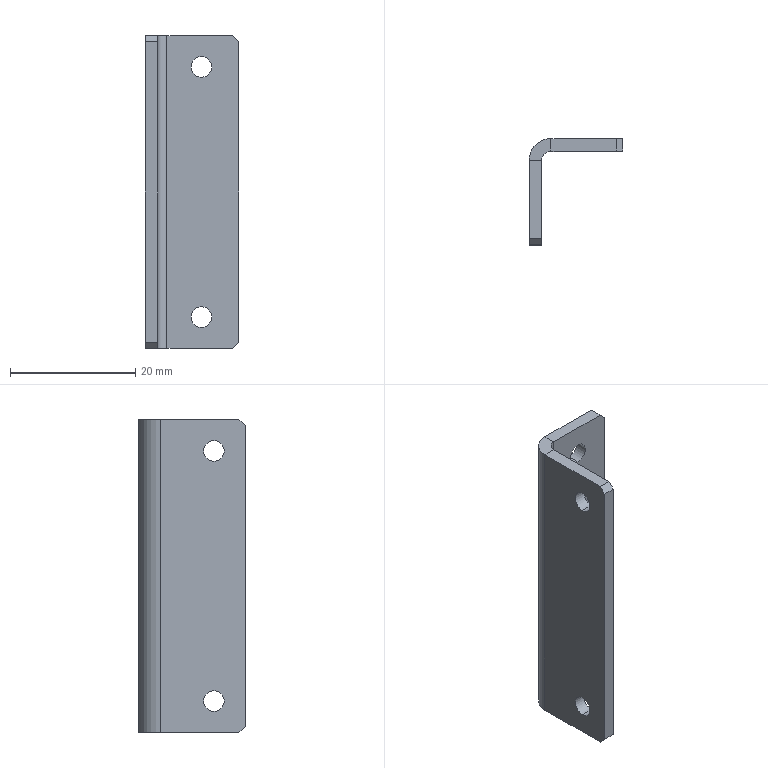Part | SolidWorks | features HoleWzd 2, Chamfer 1, FlatPattern 1, SMBaseFlange 1, SheetMetal 1 | 1 solid | 26 faces | box 15 x 17 x 50 mm | volume 2820 mm3 | plane 16 | cylinder 10 | commonest cylinder face diameters 3.3 x8 3 x1 7 x1
STEP:
#1=CARTESIAN_POINT('',(2.,5.,18.35));
#2=VERTEX_POINT('',#1);
#3=CARTESIAN_POINT('',(2.,5.,21.65));
#4=VERTEX_POINT('',#3);
#5=CARTESIAN_POINT('',(2.,5.,20.));
#6=DIRECTION('',(-1.,0.,0.));
#7=DIRECTION('',(0.,0.,1.));
#8=AXIS2_PLACEMENT_3D('',#5,#6,#7);
#9=CIRCLE('',#8,1.65);
#10=EDGE_CURVE('',#2,#4,#9,.T.);
#11=ORIENTED_EDGE('',*,*,#10,.F.);
#12=CARTESIAN_POINT('',(0.,5.,18.35));
#13=VERTEX_POINT('',#12);
#14=CARTESIAN_POINT('',(0.,5.,18.35));
#15=DIRECTION('',(-1.,0.,0.));
#16=VECTOR('',#15,1000.);
#17=LINE('',#14,#16);
#18=EDGE_CURVE('',#2,#13,#17,.T.);
#19=ORIENTED_EDGE('',*,*,#18,.T.);
#20=CARTESIAN_POINT('',(0.,5.,21.65));
#21=VERTEX_POINT('',#20);
#22=CARTESIAN_POINT('',(0.,5.,20.));
#23=DIRECTION('',(-1.,0.,0.));
#24=DIRECTION('',(0.,0.,1.));
#25=AXIS2_PLACEMENT_3D('',#22,#23,#24);
#26=CIRCLE('',#25,1.65);
#27=EDGE_CURVE('',#13,#21,#26,.T.);
#28=ORIENTED_EDGE('',*,*,#27,.T.);
#29=CARTESIAN_POINT('',(0.,5.,21.65));
#30=DIRECTION('',(-1.,0.,0.));
#31=VECTOR('',#30,1000.);
#32=LINE('',#29,#31);
#33=EDGE_CURVE('',#4,#21,#32,.T.);
#34=ORIENTED_EDGE('',*,*,#33,.F.);
#35=EDGE_LOOP('',(#11,#19,#28,#34));
#36=FACE_OUTER_BOUND('',#35,.T.);
#37=CARTESIAN_POINT('',(0.,5.,20.));
#38=DIRECTION('',(-1.,0.,0.));
#39=DIRECTION('',(0.,0.,1.));
#40=AXIS2_PLACEMENT_3D('',#37,#38,#39);
#41=CYLINDRICAL_SURFACE('',#40,1.65);
#42=ADVANCED_FACE('',(#36),#41,.F.);
#43=CARTESIAN_POINT('',(2.,5.,-21.65));
#44=VERTEX_POINT('',#43);
#45=CARTESIAN_POINT('',(2.,5.,-18.35));
#46=VERTEX_POINT('',#45);
#47=CARTESIAN_POINT('',(2.,5.,-20.));
#48=DIRECTION('',(-1.,0.,0.));
#49=DIRECTION('',(0.,0.,1.));
#50=AXIS2_PLACEMENT_3D('',#47,#48,#49);
#51=CIRCLE('',#50,1.65);
#52=EDGE_CURVE('',#44,#46,#51,.T.);
#53=ORIENTED_EDGE('',*,*,#52,.F.);
#54=CARTESIAN_POINT('',(0.,5.,-21.65));
#55=VERTEX_POINT('',#54);
#56=CARTESIAN_POINT('',(0.,5.,-21.65));
#57=DIRECTION('',(-1.,0.,0.));
#58=VECTOR('',#57,1000.);
#59=LINE('',#56,#58);
#60=EDGE_CURVE('',#44,#55,#59,.T.);
#61=ORIENTED_EDGE('',*,*,#60,.T.);
#62=CARTESIAN_POINT('',(0.,5.,-18.35));
#63=VERTEX_POINT('',#62);
#64=CARTESIAN_POINT('',(0.,5.,-20.));
#65=DIRECTION('',(-1.,0.,0.));
#66=DIRECTION('',(0.,0.,1.));
#67=AXIS2_PLACEMENT_3D('',#64,#65,#66);
#68=CIRCLE('',#67,1.65);
#69=EDGE_CURVE('',#55,#63,#68,.T.);
#70=ORIENTED_EDGE('',*,*,#69,.T.);
#71=CARTESIAN_POINT('',(0.,5.,-18.35));
#72=DIRECTION('',(-1.,0.,0.));
#73=VECTOR('',#72,1000.);
#74=LINE('',#71,#73);
#75=EDGE_CURVE('',#46,#63,#74,.T.);
#76=ORIENTED_EDGE('',*,*,#75,.F.);
#77=EDGE_LOOP('',(#53,#61,#70,#76));
#78=FACE_OUTER_BOUND('',#77,.T.);
#79=CARTESIAN_POINT('',(0.,5.,-20.));
#80=DIRECTION('',(-1.,0.,0.));
#81=DIRECTION('',(0.,0.,1.));
#82=AXIS2_PLACEMENT_3D('',#79,#80,#81);
#83=CYLINDRICAL_SURFACE('',#82,1.65);
#84=ADVANCED_FACE('',(#78),#83,.F.);
#85=CARTESIAN_POINT('',(9.,15.,-21.65));
#86=VERTEX_POINT('',#85);
#87=CARTESIAN_POINT('',(9.,15.,-18.35));
#88=VERTEX_POINT('',#87);
#89=CARTESIAN_POINT('',(9.,15.,-20.));
#90=DIRECTION('',(0.,1.,0.));
#91=DIRECTION('',(0.,0.,1.));
#92=AXIS2_PLACEMENT_3D('',#89,#90,#91);
#93=CIRCLE('',#92,1.65);
#94=EDGE_CURVE('',#86,#88,#93,.T.);
#95=ORIENTED_EDGE('',*,*,#94,.F.);
#96=CARTESIAN_POINT('',(9.,17.,-21.65));
#97=VERTEX_POINT('',#96);
#98=CARTESIAN_POINT('',(9.,17.,-21.65));
#99=DIRECTION('',(0.,1.,0.));
#100=VECTOR('',#99,1000.);
#101=LINE('',#98,#100);
#102=EDGE_CURVE('',#86,#97,#101,.T.);
#103=ORIENTED_EDGE('',*,*,#102,.T.);
#104=CARTESIAN_POINT('',(9.,17.,-18.35));
#105=VERTEX_POINT('',#104);
#106=CARTESIAN_POINT('',(9.,17.,-20.));
#107=DIRECTION('',(0.,1.,0.));
#108=DIRECTION('',(0.,0.,1.));
#109=AXIS2_PLACEMENT_3D('',#106,#107,#108);
#110=CIRCLE('',#109,1.65);
#111=EDGE_CURVE('',#97,#105,#110,.T.);
#112=ORIENTED_EDGE('',*,*,#111,.T.);
#113=CARTESIAN_POINT('',(9.,17.,-18.35));
#114=DIRECTION('',(0.,1.,0.));
#115=VECTOR('',#114,1000.);
#116=LINE('',#113,#115);
#117=EDGE_CURVE('',#88,#105,#116,.T.);
#118=ORIENTED_EDGE('',*,*,#117,.F.);
#119=EDGE_LOOP('',(#95,#103,#112,#118));
#120=FACE_OUTER_BOUND('',#119,.T.);
#121=CARTESIAN_POINT('',(9.,17.,-20.));
#122=DIRECTION('',(0.,1.,0.));
#123=DIRECTION('',(0.,0.,1.));
#124=AXIS2_PLACEMENT_3D('',#121,#122,#123);
#125=CYLINDRICAL_SURFACE('',#124,1.65);
#126=ADVANCED_FACE('',(#120),#125,.F.);
#127=CARTESIAN_POINT('',(9.,15.,18.35));
#128=VERTEX_POINT('',#127);
#129=CARTESIAN_POINT('',(9.,15.,21.65));
#130=VERTEX_POINT('',#129);
#131=CARTESIAN_POINT('',(9.,15.,20.));
#132=DIRECTION('',(0.,1.,0.));
#133=DIRECTION('',(0.,0.,1.));
#134=AXIS2_PLACEMENT_3D('',#131,#132,#133);
#135=CIRCLE('',#134,1.65);
#136=EDGE_CURVE('',#128,#130,#135,.T.);
#137=ORIENTED_EDGE('',*,*,#136,.F.);
#138=CARTESIAN_POINT('',(9.,17.,18.35));
#139=VERTEX_POINT('',#138);
#140=CARTESIAN_POINT('',(9.,17.,18.35));
#141=DIRECTION('',(0.,1.,0.));
#142=VECTOR('',#141,1000.);
#143=LINE('',#140,#142);
#144=EDGE_CURVE('',#128,#139,#143,.T.);
#145=ORIENTED_EDGE('',*,*,#144,.T.);
#146=CARTESIAN_POINT('',(9.,17.,21.65));
#147=VERTEX_POINT('',#146);
#148=CARTESIAN_POINT('',(9.,17.,20.));
#149=DIRECTION('',(0.,1.,0.));
#150=DIRECTION('',(0.,0.,1.));
#151=AXIS2_PLACEMENT_3D('',#148,#149,#150);
#152=CIRCLE('',#151,1.65);
#153=EDGE_CURVE('',#139,#147,#152,.T.);
#154=ORIENTED_EDGE('',*,*,#153,.T.);
#155=CARTESIAN_POINT('',(9.,17.,21.65));
#156=DIRECTION('',(0.,1.,0.));
#157=VECTOR('',#156,1000.);
#158=LINE('',#155,#157);
#159=EDGE_CURVE('',#130,#147,#158,.T.);
#160=ORIENTED_EDGE('',*,*,#159,.F.);
#161=EDGE_LOOP('',(#137,#145,#154,#160));
#162=FACE_OUTER_BOUND('',#161,.T.);
#163=CARTESIAN_POINT('',(9.,17.,20.));
#164=DIRECTION('',(0.,1.,0.));
#165=DIRECTION('',(0.,0.,1.));
#166=AXIS2_PLACEMENT_3D('',#163,#164,#165);
#167=CYLINDRICAL_SURFACE('',#166,1.65);
#168=ADVANCED_FACE('',(#162),#167,.F.);
#169=CARTESIAN_POINT('',(3.5,17.,25.));
#170=VERTEX_POINT('',#169);
#171=CARTESIAN_POINT('',(3.5,15.,25.));
#172=VERTEX_POINT('',#171);
#173=CARTESIAN_POINT('',(3.5,17.,25.));
#174=DIRECTION('',(0.,-1.,0.));
#175=VECTOR('',#174,1000.);
#176=LINE('',#173,#175);
#177=EDGE_CURVE('',#170,#172,#176,.T.);
#178=ORIENTED_EDGE('',*,*,#177,.F.);
#179=CARTESIAN_POINT('',(0.,13.5,25.));
#180=VERTEX_POINT('',#179);
#181=CARTESIAN_POINT('',(3.5,13.5,25.));
#182=DIRECTION('',(0.,0.,-1.));
#183=DIRECTION('',(1.,0.,0.));
#184=AXIS2_PLACEMENT_3D('',#181,#182,#183);
#185=CIRCLE('',#184,3.5);
#186=EDGE_CURVE('',#180,#170,#185,.T.);
#187=ORIENTED_EDGE('',*,*,#186,.F.);
#188=CARTESIAN_POINT('',(2.,13.5,25.));
#189=VERTEX_POINT('',#188);
#190=CARTESIAN_POINT('',(2.,13.5,25.));
#191=DIRECTION('',(-1.,0.,0.));
#192=VECTOR('',#191,1000.);
#193=LINE('',#190,#192);
#194=EDGE_CURVE('',#189,#180,#193,.T.);
#195=ORIENTED_EDGE('',*,*,#194,.F.);
#196=CARTESIAN_POINT('',(3.5,13.5,25.));
#197=DIRECTION('',(0.,0.,-1.));
#198=DIRECTION('',(1.,0.,0.));
#199=AXIS2_PLACEMENT_3D('',#196,#197,#198);
#200=CIRCLE('',#199,1.5);
#201=EDGE_CURVE('',#189,#172,#200,.T.);
#202=ORIENTED_EDGE('',*,*,#201,.T.);
#203=EDGE_LOOP('',(#178,#187,#195,#202));
#204=FACE_OUTER_BOUND('',#203,.T.);
#205=CARTESIAN_POINT('',(3.5,17.,25.));
#206=DIRECTION('',(0.,0.,1.));
#207=DIRECTION('',(1.,0.,0.));
#208=AXIS2_PLACEMENT_3D('',#205,#206,#207);
#209=PLANE('',#208);
#210=ADVANCED_FACE('',(#204),#209,.T.);
#211=CARTESIAN_POINT('',(14.,15.,25.));
#212=VERTEX_POINT('',#211);
#213=CARTESIAN_POINT('',(0.,15.,25.));
#214=DIRECTION('',(1.,0.,0.));
#215=VECTOR('',#214,1000.);
#216=LINE('',#213,#215);
#217=EDGE_CURVE('',#172,#212,#216,.T.);
#218=ORIENTED_EDGE('',*,*,#217,.T.);
#219=CARTESIAN_POINT('',(14.,17.,25.));
#220=VERTEX_POINT('',#219);
#221=CARTESIAN_POINT('',(14.,13.5,25.));
#222=DIRECTION('',(0.,1.,0.));
#223=VECTOR('',#222,1000.);
#224=LINE('',#221,#223);
#225=EDGE_CURVE('',#212,#220,#224,.T.);
#226=ORIENTED_EDGE('',*,*,#225,.T.);
#227=CARTESIAN_POINT('',(0.,17.,25.));
#228=DIRECTION('',(1.,0.,0.));
#229=VECTOR('',#228,1000.);
#230=LINE('',#227,#229);
#231=EDGE_CURVE('',#170,#220,#230,.T.);
#232=ORIENTED_EDGE('',*,*,#231,.F.);
#233=ORIENTED_EDGE('',*,*,#177,.T.);
#234=EDGE_LOOP('',(#218,#226,#232,#233));
#235=FACE_OUTER_BOUND('',#234,.T.);
#236=CARTESIAN_POINT('',(2.,13.5,25.));
#237=DIRECTION('',(0.,0.,1.));
#238=DIRECTION('',(1.,0.,0.));
#239=AXIS2_PLACEMENT_3D('',#236,#237,#238);
#240=PLANE('',#239);
#241=ADVANCED_FACE('',(#235),#240,.T.);
#242=CARTESIAN_POINT('',(0.,13.5,-25.));
#243=VERTEX_POINT('',#242);
#244=CARTESIAN_POINT('',(2.,13.5,-25.));
#245=VERTEX_POINT('',#244);
#246=CARTESIAN_POINT('',(0.,13.5,-25.));
#247=DIRECTION('',(1.,0.,0.));
#248=VECTOR('',#247,1000.);
#249=LINE('',#246,#248);
#250=EDGE_CURVE('',#243,#245,#249,.T.);
#251=ORIENTED_EDGE('',*,*,#250,.F.);
#252=CARTESIAN_POINT('',(3.5,17.,-25.));
#253=VERTEX_POINT('',#252);
#254=CARTESIAN_POINT('',(3.5,13.5,-25.));
#255=DIRECTION('',(0.,0.,-1.));
#256=DIRECTION('',(1.,0.,0.));
#257=AXIS2_PLACEMENT_3D('',#254,#255,#256);
#258=CIRCLE('',#257,3.5);
#259=EDGE_CURVE('',#243,#253,#258,.T.);
#260=ORIENTED_EDGE('',*,*,#259,.T.);
#261=CARTESIAN_POINT('',(3.5,15.,-25.));
#262=VERTEX_POINT('',#261);
#263=CARTESIAN_POINT('',(3.5,15.,-25.));
#264=DIRECTION('',(0.,1.,0.));
#265=VECTOR('',#264,1000.);
#266=LINE('',#263,#265);
#267=EDGE_CURVE('',#262,#253,#266,.T.);
#268=ORIENTED_EDGE('',*,*,#267,.F.);
#269=CARTESIAN_POINT('',(3.5,13.5,-25.));
#270=DIRECTION('',(0.,0.,-1.));
#271=DIRECTION('',(1.,0.,0.));
#272=AXIS2_PLACEMENT_3D('',#269,#270,#271);
#273=CIRCLE('',#272,1.5);
#274=EDGE_CURVE('',#245,#262,#273,.T.);
#275=ORIENTED_EDGE('',*,*,#274,.F.);
#276=EDGE_LOOP('',(#251,#260,#268,#275));
#277=FACE_OUTER_BOUND('',#276,.T.);
#278=CARTESIAN_POINT('',(0.,13.5,-25.));
#279=DIRECTION('',(0.,0.,-1.));
#280=DIRECTION('',(-1.,0.,0.));
#281=AXIS2_PLACEMENT_3D('',#278,#279,#280);
#282=PLANE('',#281);
#283=ADVANCED_FACE('',(#277),#282,.T.);
#284=CARTESIAN_POINT('',(2.,1.,-25.));
#285=VERTEX_POINT('',#284);
#286=CARTESIAN_POINT('',(2.,0.,-25.));
#287=DIRECTION('',(0.,1.,0.));
#288=VECTOR('',#287,1000.);
#289=LINE('',#286,#288);
#290=EDGE_CURVE('',#285,#245,#289,.T.);
#291=ORIENTED_EDGE('',*,*,#290,.F.);
#292=CARTESIAN_POINT('',(0.,1.,-25.));
#293=VERTEX_POINT('',#292);
#294=CARTESIAN_POINT('',(3.5,1.,-25.));
#295=DIRECTION('',(-1.,0.,0.));
#296=VECTOR('',#295,1000.);
#297=LINE('',#294,#296);
#298=EDGE_CURVE('',#285,#293,#297,.T.);
#299=ORIENTED_EDGE('',*,*,#298,.T.);
#300=CARTESIAN_POINT('',(0.,0.,-25.));
#301=DIRECTION('',(0.,1.,0.));
#302=VECTOR('',#301,1000.);
#303=LINE('',#300,#302);
#304=EDGE_CURVE('',#293,#243,#303,.T.);
#305=ORIENTED_EDGE('',*,*,#304,.T.);
#306=ORIENTED_EDGE('',*,*,#250,.T.);
#307=EDGE_LOOP('',(#291,#299,#305,#306));
#308=FACE_OUTER_BOUND('',#307,.T.);
#309=CARTESIAN_POINT('',(3.5,15.,-25.));
#310=DIRECTION('',(0.,0.,-1.));
#311=DIRECTION('',(-1.,0.,0.));
#312=AXIS2_PLACEMENT_3D('',#309,#310,#311);
#313=PLANE('',#312);
#314=ADVANCED_FACE('',(#308),#313,.T.);
#315=CARTESIAN_POINT('',(9.,15.,-20.));
#316=DIRECTION('',(0.,1.,0.));
#317=DIRECTION('',(0.,0.,1.));
#318=AXIS2_PLACEMENT_3D('',#315,#316,#317);
#319=CIRCLE('',#318,1.65);
#320=EDGE_CURVE('',#88,#86,#319,.T.);
#321=ORIENTED_EDGE('',*,*,#320,.T.);
#322=ORIENTED_EDGE('',*,*,#94,.T.);
#323=EDGE_LOOP('',(#321,#322));
#324=FACE_BOUND('',#323,.T.);
#325=CARTESIAN_POINT('',(9.,15.,20.));
#326=DIRECTION('',(0.,1.,0.));
#327=DIRECTION('',(0.,0.,1.));
#328=AXIS2_PLACEMENT_3D('',#325,#326,#327);
#329=CIRCLE('',#328,1.65);
#330=EDGE_CURVE('',#130,#128,#329,.T.);
#331=ORIENTED_EDGE('',*,*,#330,.T.);
#332=ORIENTED_EDGE('',*,*,#136,.T.);
#333=EDGE_LOOP('',(#331,#332));
#334=FACE_BOUND('',#333,.T.);
#335=CARTESIAN_POINT('',(14.,15.,-25.));
#336=VERTEX_POINT('',#335);
#337=CARTESIAN_POINT('',(0.,15.,-25.));
#338=DIRECTION('',(1.,0.,0.));
#339=VECTOR('',#338,1000.);
#340=LINE('',#337,#339);
#341=EDGE_CURVE('',#262,#336,#340,.T.);
#342=ORIENTED_EDGE('',*,*,#341,.T.);
#343=CARTESIAN_POINT('',(15.,15.,-24.));
#344=VERTEX_POINT('',#343);
#345=CARTESIAN_POINT('',(14.,15.,-25.));
#346=DIRECTION('',(0.7071,0.,0.7071));
#347=VECTOR('',#346,1000.);
#348=LINE('',#345,#347);
#349=EDGE_CURVE('',#336,#344,#348,.T.);
#350=ORIENTED_EDGE('',*,*,#349,.T.);
#351=CARTESIAN_POINT('',(15.,15.,24.));
#352=VERTEX_POINT('',#351);
#353=CARTESIAN_POINT('',(15.,15.,25.));
#354=DIRECTION('',(0.,0.,-1.));
#355=VECTOR('',#354,1000.);
#356=LINE('',#353,#355);
#357=EDGE_CURVE('',#352,#344,#356,.T.);
#358=ORIENTED_EDGE('',*,*,#357,.F.);
#359=CARTESIAN_POINT('',(15.,15.,24.));
#360=DIRECTION('',(-0.7071,0.,0.7071));
#361=VECTOR('',#360,1000.);
#362=LINE('',#359,#361);
#363=EDGE_CURVE('',#352,#212,#362,.T.);
#364=ORIENTED_EDGE('',*,*,#363,.T.);
#365=ORIENTED_EDGE('',*,*,#217,.F.);
#366=CARTESIAN_POINT('',(3.5,15.,25.));
#367=DIRECTION('',(0.,0.,-1.));
#368=VECTOR('',#367,1000.);
#369=LINE('',#366,#368);
#370=EDGE_CURVE('',#172,#262,#369,.T.);
#371=ORIENTED_EDGE('',*,*,#370,.T.);
#372=EDGE_LOOP('',(#342,#350,#358,#364,#365,#371));
#373=FACE_OUTER_BOUND('',#372,.T.);
#374=CARTESIAN_POINT('',(0.,15.,25.));
#375=DIRECTION('',(0.,1.,0.));
#376=DIRECTION('',(0.,0.,1.));
#377=AXIS2_PLACEMENT_3D('',#374,#375,#376);
#378=PLANE('',#377);
#379=ADVANCED_FACE('',(#324,#334,#373),#378,.F.);
#380=ORIENTED_EDGE('',*,*,#357,.T.);
#381=CARTESIAN_POINT('',(15.,17.,-24.));
#382=VERTEX_POINT('',#381);
#383=CARTESIAN_POINT('',(15.,17.,-24.));
#384=DIRECTION('',(0.,1.,0.));
#385=VECTOR('',#384,1000.);
#386=LINE('',#383,#385);
#387=EDGE_CURVE('',#344,#382,#386,.T.);
#388=ORIENTED_EDGE('',*,*,#387,.T.);
#389=CARTESIAN_POINT('',(15.,17.,24.));
#390=VERTEX_POINT('',#389);
#391=CARTESIAN_POINT('',(15.,17.,25.));
#392=DIRECTION('',(0.,0.,-1.));
#393=VECTOR('',#392,1000.);
#394=LINE('',#391,#393);
#395=EDGE_CURVE('',#390,#382,#394,.T.);
#396=ORIENTED_EDGE('',*,*,#395,.F.);
#397=CARTESIAN_POINT('',(15.,17.,24.));
#398=DIRECTION('',(0.,-1.,0.));
#399=VECTOR('',#398,1000.);
#400=LINE('',#397,#399);
#401=EDGE_CURVE('',#390,#352,#400,.T.);
#402=ORIENTED_EDGE('',*,*,#401,.T.);
#403=EDGE_LOOP('',(#380,#388,#396,#402));
#404=FACE_OUTER_BOUND('',#403,.T.);
#405=CARTESIAN_POINT('',(15.,17.,25.));
#406=DIRECTION('',(1.,0.,0.));
#407=DIRECTION('',(0.,0.,-1.));
#408=AXIS2_PLACEMENT_3D('',#405,#406,#407);
#409=PLANE('',#408);
#410=ADVANCED_FACE('',(#404),#409,.T.);
#411=CARTESIAN_POINT('',(9.,17.,-20.));
#412=DIRECTION('',(0.,1.,0.));
#413=DIRECTION('',(0.,0.,1.));
#414=AXIS2_PLACEMENT_3D('',#411,#412,#413);
#415=CIRCLE('',#414,1.65);
#416=EDGE_CURVE('',#105,#97,#415,.T.);
#417=ORIENTED_EDGE('',*,*,#416,.F.);
#418=ORIENTED_EDGE('',*,*,#111,.F.);
#419=EDGE_LOOP('',(#417,#418));
#420=FACE_BOUND('',#419,.T.);
#421=CARTESIAN_POINT('',(9.,17.,20.));
#422=DIRECTION('',(0.,1.,0.));
#423=DIRECTION('',(0.,0.,1.));
#424=AXIS2_PLACEMENT_3D('',#421,#422,#423);
#425=CIRCLE('',#424,1.65);
#426=EDGE_CURVE('',#147,#139,#425,.T.);
#427=ORIENTED_EDGE('',*,*,#426,.F.);
#428=ORIENTED_EDGE('',*,*,#153,.F.);
#429=EDGE_LOOP('',(#427,#428));
#430=FACE_BOUND('',#429,.T.);
#431=ORIENTED_EDGE('',*,*,#395,.T.);
#432=CARTESIAN_POINT('',(14.,17.,-25.));
#433=VERTEX_POINT('',#432);
#434=CARTESIAN_POINT('',(32.,17.,-7.));
#435=DIRECTION('',(-0.7071,0.,-0.7071));
#436=VECTOR('',#435,1000.);
#437=LINE('',#434,#436);
#438=EDGE_CURVE('',#382,#433,#437,.T.);
#439=ORIENTED_EDGE('',*,*,#438,.T.);
#440=CARTESIAN_POINT('',(0.,17.,-25.));
#441=DIRECTION('',(1.,0.,0.));
#442=VECTOR('',#441,1000.);
#443=LINE('',#440,#442);
#444=EDGE_CURVE('',#253,#433,#443,.T.);
#445=ORIENTED_EDGE('',*,*,#444,.F.);
#446=CARTESIAN_POINT('',(3.5,17.,25.));
#447=DIRECTION('',(0.,0.,-1.));
#448=VECTOR('',#447,1000.);
#449=LINE('',#446,#448);
#450=EDGE_CURVE('',#170,#253,#449,.T.);
#451=ORIENTED_EDGE('',*,*,#450,.F.);
#452=ORIENTED_EDGE('',*,*,#231,.T.);
#453=CARTESIAN_POINT('',(7.,17.,32.));
#454=DIRECTION('',(0.7071,0.,-0.7071));
#455=VECTOR('',#454,1000.);
#456=LINE('',#453,#455);
#457=EDGE_CURVE('',#220,#390,#456,.T.);
#458=ORIENTED_EDGE('',*,*,#457,.T.);
#459=EDGE_LOOP('',(#431,#439,#445,#451,#452,#458));
#460=FACE_OUTER_BOUND('',#459,.T.);
#461=CARTESIAN_POINT('',(0.,17.,25.));
#462=DIRECTION('',(0.,1.,0.));
#463=DIRECTION('',(0.,0.,1.));
#464=AXIS2_PLACEMENT_3D('',#461,#462,#463);
#465=PLANE('',#464);
#466=ADVANCED_FACE('',(#420,#430,#460),#465,.T.);
#467=ORIENTED_EDGE('',*,*,#259,.F.);
#468=CARTESIAN_POINT('',(0.,13.5,25.));
#469=DIRECTION('',(0.,0.,-1.));
#470=VECTOR('',#469,1000.);
#471=LINE('',#468,#470);
#472=EDGE_CURVE('',#180,#243,#471,.T.);
#473=ORIENTED_EDGE('',*,*,#472,.F.);
#474=ORIENTED_EDGE('',*,*,#186,.T.);
#475=ORIENTED_EDGE('',*,*,#450,.T.);
#476=EDGE_LOOP('',(#467,#473,#474,#475));
#477=FACE_OUTER_BOUND('',#476,.T.);
#478=CARTESIAN_POINT('',(3.5,13.5,25.));
#479=DIRECTION('',(0.,0.,-1.));
#480=DIRECTION('',(-1.,0.,0.));
#481=AXIS2_PLACEMENT_3D('',#478,#479,#480);
#482=CYLINDRICAL_SURFACE('',#481,3.5);
#483=ADVANCED_FACE('',(#477),#482,.T.);
#484=CARTESIAN_POINT('',(0.,5.,20.));
#485=DIRECTION('',(-1.,0.,0.));
#486=DIRECTION('',(0.,0.,1.));
#487=AXIS2_PLACEMENT_3D('',#484,#485,#486);
#488=CIRCLE('',#487,1.65);
#489=EDGE_CURVE('',#21,#13,#488,.T.);
#490=ORIENTED_EDGE('',*,*,#489,.F.);
#491=ORIENTED_EDGE('',*,*,#27,.F.);
#492=EDGE_LOOP('',(#490,#491));
#493=FACE_BOUND('',#492,.T.);
#494=CARTESIAN_POINT('',(0.,5.,-20.));
#495=DIRECTION('',(-1.,0.,0.));
#496=DIRECTION('',(0.,0.,1.));
#497=AXIS2_PLACEMENT_3D('',#494,#495,#496);
#498=CIRCLE('',#497,1.65);
#499=EDGE_CURVE('',#63,#55,#498,.T.);
#500=ORIENTED_EDGE('',*,*,#499,.F.);
#501=ORIENTED_EDGE('',*,*,#69,.F.);
#502=EDGE_LOOP('',(#500,#501));
#503=FACE_BOUND('',#502,.T.);
#504=ORIENTED_EDGE('',*,*,#304,.F.);
#505=CARTESIAN_POINT('',(0.,0.,-24.));
#506=VERTEX_POINT('',#505);
#507=CARTESIAN_POINT('',(0.,-24.5,0.5));
#508=DIRECTION('',(0.,-0.7071,0.7071));
#509=VECTOR('',#508,1000.);
#510=LINE('',#507,#509);
#511=EDGE_CURVE('',#293,#506,#510,.T.);
#512=ORIENTED_EDGE('',*,*,#511,.T.);
#513=CARTESIAN_POINT('',(0.,0.,24.));
#514=VERTEX_POINT('',#513);
#515=CARTESIAN_POINT('',(0.,0.,25.));
#516=DIRECTION('',(0.,0.,-1.));
#517=VECTOR('',#516,1000.);
#518=LINE('',#515,#517);
#519=EDGE_CURVE('',#514,#506,#518,.T.);
#520=ORIENTED_EDGE('',*,*,#519,.F.);
#521=CARTESIAN_POINT('',(0.,1.,25.));
#522=VERTEX_POINT('',#521);
#523=CARTESIAN_POINT('',(0.,0.5,24.5));
#524=DIRECTION('',(0.,0.7071,0.7071));
#525=VECTOR('',#524,1000.);
#526=LINE('',#523,#525);
#527=EDGE_CURVE('',#514,#522,#526,.T.);
#528=ORIENTED_EDGE('',*,*,#527,.T.);
#529=CARTESIAN_POINT('',(0.,0.,25.));
#530=DIRECTION('',(0.,1.,0.));
#531=VECTOR('',#530,1000.);
#532=LINE('',#529,#531);
#533=EDGE_CURVE('',#522,#180,#532,.T.);
#534=ORIENTED_EDGE('',*,*,#533,.T.);
#535=ORIENTED_EDGE('',*,*,#472,.T.);
#536=EDGE_LOOP('',(#504,#512,#520,#528,#534,#535));
#537=FACE_OUTER_BOUND('',#536,.T.);
#538=CARTESIAN_POINT('',(0.,0.,25.));
#539=DIRECTION('',(-1.,0.,0.));
#540=DIRECTION('',(0.,0.,1.));
#541=AXIS2_PLACEMENT_3D('',#538,#539,#540);
#542=PLANE('',#541);
#543=ADVANCED_FACE('',(#493,#503,#537),#542,.T.);
#544=ORIENTED_EDGE('',*,*,#519,.T.);
#545=CARTESIAN_POINT('',(2.,0.,-24.));
#546=VERTEX_POINT('',#545);
#547=CARTESIAN_POINT('',(2.,0.,-24.));
#548=DIRECTION('',(1.,0.,0.));
#549=VECTOR('',#548,1000.);
#550=LINE('',#547,#549);
#551=EDGE_CURVE('',#506,#546,#550,.T.);
#552=ORIENTED_EDGE('',*,*,#551,.T.);
#553=CARTESIAN_POINT('',(2.,0.,24.));
#554=VERTEX_POINT('',#553);
#555=CARTESIAN_POINT('',(2.,0.,25.));
#556=DIRECTION('',(0.,0.,-1.));
#557=VECTOR('',#556,1000.);
#558=LINE('',#555,#557);
#559=EDGE_CURVE('',#554,#546,#558,.T.);
#560=ORIENTED_EDGE('',*,*,#559,.F.);
#561=CARTESIAN_POINT('',(2.,0.,24.));
#562=DIRECTION('',(-1.,0.,0.));
#563=VECTOR('',#562,1000.);
#564=LINE('',#561,#563);
#565=EDGE_CURVE('',#554,#514,#564,.T.);
#566=ORIENTED_EDGE('',*,*,#565,.T.);
#567=EDGE_LOOP('',(#544,#552,#560,#566));
#568=FACE_OUTER_BOUND('',#567,.T.);
#569=CARTESIAN_POINT('',(2.,0.,25.));
#570=DIRECTION('',(0.,-1.,0.));
#571=DIRECTION('',(0.,0.,-1.));
#572=AXIS2_PLACEMENT_3D('',#569,#570,#571);
#573=PLANE('',#572);
#574=ADVANCED_FACE('',(#568),#573,.T.);
#575=CARTESIAN_POINT('',(2.,5.,20.));
#576=DIRECTION('',(-1.,0.,0.));
#577=DIRECTION('',(0.,0.,1.));
#578=AXIS2_PLACEMENT_3D('',#575,#576,#577);
#579=CIRCLE('',#578,1.65);
#580=EDGE_CURVE('',#4,#2,#579,.T.);
#581=ORIENTED_EDGE('',*,*,#580,.T.);
#582=ORIENTED_EDGE('',*,*,#10,.T.);
#583=EDGE_LOOP('',(#581,#582));
#584=FACE_BOUND('',#583,.T.);
#585=CARTESIAN_POINT('',(2.,5.,-20.));
#586=DIRECTION('',(-1.,0.,0.));
#587=DIRECTION('',(0.,0.,1.));
#588=AXIS2_PLACEMENT_3D('',#585,#586,#587);
#589=CIRCLE('',#588,1.65);
#590=EDGE_CURVE('',#46,#44,#589,.T.);
#591=ORIENTED_EDGE('',*,*,#590,.T.);
#592=ORIENTED_EDGE('',*,*,#52,.T.);
#593=EDGE_LOOP('',(#591,#592));
#594=FACE_BOUND('',#593,.T.);
#595=ORIENTED_EDGE('',*,*,#559,.T.);
#596=CARTESIAN_POINT('',(2.,1.,-25.));
#597=DIRECTION('',(0.,0.7071,-0.7071));
#598=VECTOR('',#597,1000.);
#599=LINE('',#596,#598);
#600=EDGE_CURVE('',#546,#285,#599,.T.);
#601=ORIENTED_EDGE('',*,*,#600,.T.);
#602=ORIENTED_EDGE('',*,*,#290,.T.);
#603=CARTESIAN_POINT('',(2.,13.5,25.));
#604=DIRECTION('',(0.,0.,-1.));
#605=VECTOR('',#604,1000.);
#606=LINE('',#603,#605);
#607=EDGE_CURVE('',#189,#245,#606,.T.);
#608=ORIENTED_EDGE('',*,*,#607,.F.);
#609=CARTESIAN_POINT('',(2.,1.,25.));
#610=VERTEX_POINT('',#609);
#611=CARTESIAN_POINT('',(2.,0.,25.));
#612=DIRECTION('',(0.,1.,0.));
#613=VECTOR('',#612,1000.);
#614=LINE('',#611,#613);
#615=EDGE_CURVE('',#610,#189,#614,.T.);
#616=ORIENTED_EDGE('',*,*,#615,.F.);
#617=CARTESIAN_POINT('',(2.,0.,24.));
#618=DIRECTION('',(0.,-0.7071,-0.7071));
#619=VECTOR('',#618,1000.);
#620=LINE('',#617,#619);
#621=EDGE_CURVE('',#610,#554,#620,.T.);
#622=ORIENTED_EDGE('',*,*,#621,.T.);
#623=EDGE_LOOP('',(#595,#601,#602,#608,#616,#622));
#624=FACE_OUTER_BOUND('',#623,.T.);
#625=CARTESIAN_POINT('',(2.,0.,25.));
#626=DIRECTION('',(-1.,0.,0.));
#627=DIRECTION('',(0.,0.,1.));
#628=AXIS2_PLACEMENT_3D('',#625,#626,#627);
#629=PLANE('',#628);
#630=ADVANCED_FACE('',(#584,#594,#624),#629,.F.);
#631=ORIENTED_EDGE('',*,*,#274,.T.);
#632=ORIENTED_EDGE('',*,*,#370,.F.);
#633=ORIENTED_EDGE('',*,*,#201,.F.);
#634=ORIENTED_EDGE('',*,*,#607,.T.);
#635=EDGE_LOOP('',(#631,#632,#633,#634));
#636=FACE_OUTER_BOUND('',#635,.T.);
#637=CARTESIAN_POINT('',(3.5,13.5,25.));
#638=DIRECTION('',(0.,0.,-1.));
#639=DIRECTION('',(-1.,0.,0.));
#640=AXIS2_PLACEMENT_3D('',#637,#638,#639);
#641=CYLINDRICAL_SURFACE('',#640,1.5);
#642=ADVANCED_FACE('',(#636),#641,.F.);
#643=ORIENTED_EDGE('',*,*,#533,.F.);
#644=CARTESIAN_POINT('',(3.5,1.,25.));
#645=DIRECTION('',(1.,0.,0.));
#646=VECTOR('',#645,1000.);
#647=LINE('',#644,#646);
#648=EDGE_CURVE('',#522,#610,#647,.T.);
#649=ORIENTED_EDGE('',*,*,#648,.T.);
#650=ORIENTED_EDGE('',*,*,#615,.T.);
#651=ORIENTED_EDGE('',*,*,#194,.T.);
#652=EDGE_LOOP('',(#643,#649,#650,#651));
#653=FACE_OUTER_BOUND('',#652,.T.);
#654=CARTESIAN_POINT('',(3.5,13.5,25.));
#655=DIRECTION('',(0.,0.,1.));
#656=DIRECTION('',(1.,0.,0.));
#657=AXIS2_PLACEMENT_3D('',#654,#655,#656);
#658=PLANE('',#657);
#659=ADVANCED_FACE('',(#653),#658,.T.);
#660=ORIENTED_EDGE('',*,*,#444,.T.);
#661=CARTESIAN_POINT('',(14.,15.,-25.));
#662=DIRECTION('',(0.,-1.,0.));
#663=VECTOR('',#662,1000.);
#664=LINE('',#661,#663);
#665=EDGE_CURVE('',#433,#336,#664,.T.);
#666=ORIENTED_EDGE('',*,*,#665,.T.);
#667=ORIENTED_EDGE('',*,*,#341,.F.);
#668=ORIENTED_EDGE('',*,*,#267,.T.);
#669=EDGE_LOOP('',(#660,#666,#667,#668));
#670=FACE_OUTER_BOUND('',#669,.T.);
#671=CARTESIAN_POINT('',(3.5,13.5,-25.));
#672=DIRECTION('',(0.,0.,1.));
#673=DIRECTION('',(1.,0.,0.));
#674=AXIS2_PLACEMENT_3D('',#671,#672,#673);
#675=PLANE('',#674);
#676=ADVANCED_FACE('',(#670),#675,.F.);
#677=ORIENTED_EDGE('',*,*,#600,.F.);
#678=ORIENTED_EDGE('',*,*,#551,.F.);
#679=ORIENTED_EDGE('',*,*,#511,.F.);
#680=ORIENTED_EDGE('',*,*,#298,.F.);
#681=EDGE_LOOP('',(#677,#678,#679,#680));
#682=FACE_OUTER_BOUND('',#681,.T.);
#683=CARTESIAN_POINT('',(3.5,1.,-25.));
#684=DIRECTION('',(0.,0.7071,0.7071));
#685=DIRECTION('',(-1.,0.,0.));
#686=AXIS2_PLACEMENT_3D('',#683,#684,#685);
#687=PLANE('',#686);
#688=ADVANCED_FACE('',(#682),#687,.F.);
#689=ORIENTED_EDGE('',*,*,#621,.F.);
#690=ORIENTED_EDGE('',*,*,#648,.F.);
#691=ORIENTED_EDGE('',*,*,#527,.F.);
#692=ORIENTED_EDGE('',*,*,#565,.F.);
#693=EDGE_LOOP('',(#689,#690,#691,#692));
#694=FACE_OUTER_BOUND('',#693,.T.);
#695=CARTESIAN_POINT('',(2.,0.,24.));
#696=DIRECTION('',(0.,0.7071,-0.7071));
#697=DIRECTION('',(-1.,0.,0.));
#698=AXIS2_PLACEMENT_3D('',#695,#696,#697);
#699=PLANE('',#698);
#700=ADVANCED_FACE('',(#694),#699,.F.);
#701=ORIENTED_EDGE('',*,*,#438,.F.);
#702=ORIENTED_EDGE('',*,*,#387,.F.);
#703=ORIENTED_EDGE('',*,*,#349,.F.);
#704=ORIENTED_EDGE('',*,*,#665,.F.);
#705=EDGE_LOOP('',(#701,#702,#703,#704));
#706=FACE_OUTER_BOUND('',#705,.T.);
#707=CARTESIAN_POINT('',(14.,13.5,-25.));
#708=DIRECTION('',(0.7071,0.,-0.7071));
#709=DIRECTION('',(0.,1.,0.));
#710=AXIS2_PLACEMENT_3D('',#707,#708,#709);
#711=PLANE('',#710);
#712=ADVANCED_FACE('',(#706),#711,.T.);
#713=ORIENTED_EDGE('',*,*,#457,.F.);
#714=ORIENTED_EDGE('',*,*,#225,.F.);
#715=ORIENTED_EDGE('',*,*,#363,.F.);
#716=ORIENTED_EDGE('',*,*,#401,.F.);
#717=EDGE_LOOP('',(#713,#714,#715,#716));
#718=FACE_OUTER_BOUND('',#717,.T.);
#719=CARTESIAN_POINT('',(15.,17.,24.));
#720=DIRECTION('',(-0.7071,0.,-0.7071));
#721=DIRECTION('',(0.,-1.,0.));
#722=AXIS2_PLACEMENT_3D('',#719,#720,#721);
#723=PLANE('',#722);
#724=ADVANCED_FACE('',(#718),#723,.F.);
#725=ORIENTED_EDGE('',*,*,#144,.F.);
#726=ORIENTED_EDGE('',*,*,#330,.F.);
#727=ORIENTED_EDGE('',*,*,#159,.T.);
#728=ORIENTED_EDGE('',*,*,#426,.T.);
#729=EDGE_LOOP('',(#725,#726,#727,#728));
#730=FACE_OUTER_BOUND('',#729,.T.);
#731=CARTESIAN_POINT('',(9.,17.,20.));
#732=DIRECTION('',(0.,1.,0.));
#733=DIRECTION('',(0.,0.,1.));
#734=AXIS2_PLACEMENT_3D('',#731,#732,#733);
#735=CYLINDRICAL_SURFACE('',#734,1.65);
#736=ADVANCED_FACE('',(#730),#735,.F.);
#737=ORIENTED_EDGE('',*,*,#102,.F.);
#738=ORIENTED_EDGE('',*,*,#320,.F.);
#739=ORIENTED_EDGE('',*,*,#117,.T.);
#740=ORIENTED_EDGE('',*,*,#416,.T.);
#741=EDGE_LOOP('',(#737,#738,#739,#740));
#742=FACE_OUTER_BOUND('',#741,.T.);
#743=CARTESIAN_POINT('',(9.,17.,-20.));
#744=DIRECTION('',(0.,1.,0.));
#745=DIRECTION('',(0.,0.,1.));
#746=AXIS2_PLACEMENT_3D('',#743,#744,#745);
#747=CYLINDRICAL_SURFACE('',#746,1.65);
#748=ADVANCED_FACE('',(#742),#747,.F.);
#749=ORIENTED_EDGE('',*,*,#60,.F.);
#750=ORIENTED_EDGE('',*,*,#590,.F.);
#751=ORIENTED_EDGE('',*,*,#75,.T.);
#752=ORIENTED_EDGE('',*,*,#499,.T.);
#753=EDGE_LOOP('',(#749,#750,#751,#752));
#754=FACE_OUTER_BOUND('',#753,.T.);
#755=CARTESIAN_POINT('',(0.,5.,-20.));
#756=DIRECTION('',(-1.,0.,0.));
#757=DIRECTION('',(0.,0.,1.));
#758=AXIS2_PLACEMENT_3D('',#755,#756,#757);
#759=CYLINDRICAL_SURFACE('',#758,1.65);
#760=ADVANCED_FACE('',(#754),#759,.F.);
#761=ORIENTED_EDGE('',*,*,#18,.F.);
#762=ORIENTED_EDGE('',*,*,#580,.F.);
#763=ORIENTED_EDGE('',*,*,#33,.T.);
#764=ORIENTED_EDGE('',*,*,#489,.T.);
#765=EDGE_LOOP('',(#761,#762,#763,#764));
#766=FACE_OUTER_BOUND('',#765,.T.);
#767=CARTESIAN_POINT('',(0.,5.,20.));
#768=DIRECTION('',(-1.,0.,0.));
#769=DIRECTION('',(0.,0.,1.));
#770=AXIS2_PLACEMENT_3D('',#767,#768,#769);
#771=CYLINDRICAL_SURFACE('',#770,1.65);
#772=ADVANCED_FACE('',(#766),#771,.F.);
#773=CLOSED_SHELL('',(#42,#84,#126,#168,#210,#241,#283,#314,#379,#410,#466,#483,#543,#574,#630,#642,#659,#676,#688,#700,#712,#724,#736,#748,#760,#772));
#774=MANIFOLD_SOLID_BREP('',#773);
#775=CARTESIAN_POINT('',(0.,0.,0.));
#776=DIRECTION('',(0.,0.,1.));
#777=DIRECTION('',(1.,0.,0.));
#778=AXIS2_PLACEMENT_3D('',#775,#776,#777);
#779=(LENGTH_UNIT()NAMED_UNIT(*)SI_UNIT(.MILLI.,.METRE.));
#780=UNCERTAINTY_MEASURE_WITH_UNIT(LENGTH_MEASURE(0.00001),#779,'','');
#781=(NAMED_UNIT(*)PLANE_ANGLE_UNIT()SI_UNIT($,.RADIAN.));
#782=(NAMED_UNIT(*)SI_UNIT($,.STERADIAN.)SOLID_ANGLE_UNIT());
#783=(GEOMETRIC_REPRESENTATION_CONTEXT(3)GLOBAL_UNCERTAINTY_ASSIGNED_CONTEXT((#780))GLOBAL_UNIT_ASSIGNED_CONTEXT((#779,#781,#782))REPRESENTATION_CONTEXT('',''));
#784=ADVANCED_BREP_SHAPE_REPRESENTATION('',(#774,#778),#783);